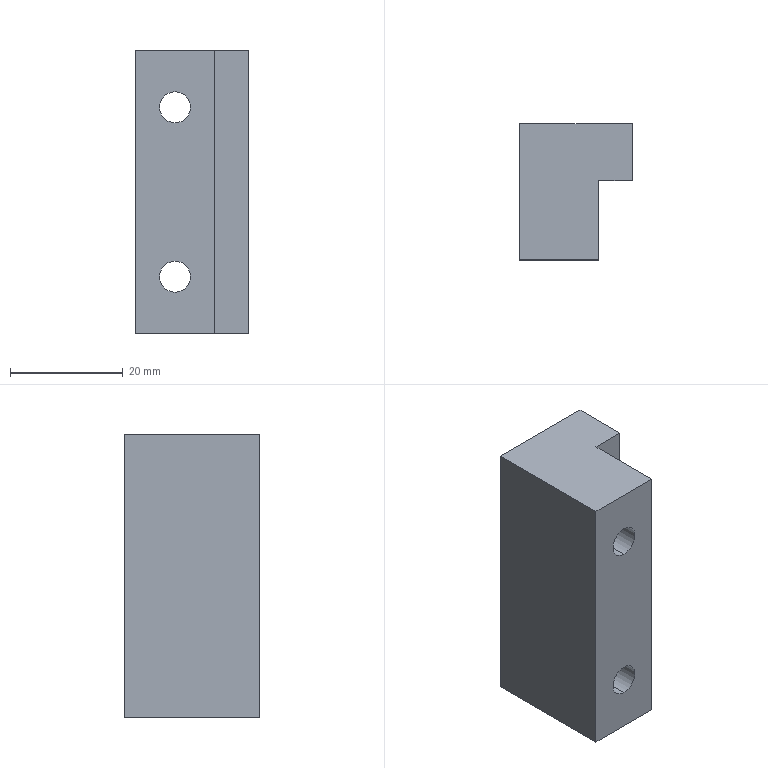Part | STEP file | Large cylinder connector mounting block | 1 solid | 18 faces | box 20 x 24 x 50 mm | volume 18141 mm3 | plane 10 | cylinder 8 | commonest cylinder face diameters 5.5 x4 9.5 x4
STEP:
#1=CARTESIAN_POINT('',(0.,0.,0.));
#2=DIRECTION('',(0.,0.,1.));
#3=DIRECTION('',(1.,0.,0.));
#4=AXIS2_PLACEMENT_3D('',#1,#2,#3);
#5=CARTESIAN_POINT('',(-13.,18.5,14.75));
#6=VERTEX_POINT('',#5);
#7=CARTESIAN_POINT('',(-13.,24.,14.75));
#8=VERTEX_POINT('',#7);
#9=CARTESIAN_POINT('',(-13.,24.,14.75));
#10=DIRECTION('',(0.,1.,0.));
#11=VECTOR('',#10,1.);
#12=LINE('',#9,#11);
#13=CARTESIAN_POINT('',(-13.,24.,10.));
#14=DIRECTION('',(0.,1.,0.));
#15=DIRECTION('',(0.,0.,1.));
#16=AXIS2_PLACEMENT_3D('',#13,#14,#15);
#17=CYLINDRICAL_SURFACE('',#16,4.75);
#18=CARTESIAN_POINT('',(6.283,0.));
#19=DIRECTION('',(0.,1.));
#20=VECTOR('',#19,1.);
#21=LINE('',#18,#20);
#22=(GEOMETRIC_REPRESENTATION_CONTEXT(2)PARAMETRIC_REPRESENTATION_CONTEXT()REPRESENTATION_CONTEXT('',''));
#23=DEFINITIONAL_REPRESENTATION('',(#21),#22);
#24=PCURVE('',#17,#23);
#25=CARTESIAN_POINT('',(-13.,24.,10.));
#26=DIRECTION('',(0.,1.,0.));
#27=DIRECTION('',(0.,0.,1.));
#28=AXIS2_PLACEMENT_3D('',#25,#26,#27);
#29=CYLINDRICAL_SURFACE('',#28,4.75);
#30=CARTESIAN_POINT('',(0.,0.));
#31=DIRECTION('',(0.,1.));
#32=VECTOR('',#31,1.);
#33=LINE('',#30,#32);
#34=(GEOMETRIC_REPRESENTATION_CONTEXT(2)PARAMETRIC_REPRESENTATION_CONTEXT()REPRESENTATION_CONTEXT('',''));
#35=DEFINITIONAL_REPRESENTATION('',(#33),#34);
#36=PCURVE('',#29,#35);
#37=SURFACE_CURVE('',#12,(#24,#36),.PCURVE_S1.);
#38=EDGE_CURVE('',#6,#8,#37,.T.);
#39=ORIENTED_EDGE('',*,*,#38,.T.);
#40=CARTESIAN_POINT('',(-13.,24.,5.25));
#41=VERTEX_POINT('',#40);
#42=CARTESIAN_POINT('',(-13.,24.,10.));
#43=DIRECTION('',(0.,1.,0.));
#44=DIRECTION('',(0.,0.,1.));
#45=AXIS2_PLACEMENT_3D('',#42,#43,#44);
#46=CIRCLE('',#45,4.75);
#47=CARTESIAN_POINT('',(0.,0.));
#48=DIRECTION('',(1.,0.));
#49=VECTOR('',#48,1.);
#50=LINE('',#47,#49);
#51=(GEOMETRIC_REPRESENTATION_CONTEXT(2)PARAMETRIC_REPRESENTATION_CONTEXT()REPRESENTATION_CONTEXT('',''));
#52=DEFINITIONAL_REPRESENTATION('',(#50),#51);
#53=PCURVE('',#17,#52);
#54=CARTESIAN_POINT('',(0.,24.,50.));
#55=DIRECTION('',(0.,-1.,0.));
#56=DIRECTION('',(1.,0.,0.));
#57=AXIS2_PLACEMENT_3D('',#54,#55,#56);
#58=PLANE('',#57);
#59=CARTESIAN_POINT('',(-13.,-35.25));
#60=CARTESIAN_POINT('',(-4.773,-35.25));
#61=CARTESIAN_POINT('',(-8.886,-42.375));
#62=CARTESIAN_POINT('',(-13.,-49.5));
#63=CARTESIAN_POINT('',(-17.114,-42.375));
#64=CARTESIAN_POINT('',(-21.227,-35.25));
#65=CARTESIAN_POINT('',(-13.,-35.25));
#66=(BOUNDED_CURVE()B_SPLINE_CURVE(2,(#59,#60,#61,#62,#63,#64,#65),.UNSPECIFIED.,.T.,.F.)B_SPLINE_CURVE_WITH_KNOTS((1,2,2,2,2,1),(-2.094,0.,2.094,4.189,6.283,8.378),.UNSPECIFIED.)CURVE()GEOMETRIC_REPRESENTATION_ITEM()RATIONAL_B_SPLINE_CURVE((1.,0.5,1.,0.5,1.,0.5,1.))REPRESENTATION_ITEM(''));
#67=(GEOMETRIC_REPRESENTATION_CONTEXT(2)PARAMETRIC_REPRESENTATION_CONTEXT()REPRESENTATION_CONTEXT('',''));
#68=DEFINITIONAL_REPRESENTATION('',(#66),#67);
#69=PCURVE('',#58,#68);
#70=SURFACE_CURVE('',#46,(#53,#69),.PCURVE_S1.);
#71=EDGE_CURVE('',#41,#8,#70,.T.);
#72=ORIENTED_EDGE('',*,*,#71,.F.);
#73=CARTESIAN_POINT('',(-13.,18.5,5.25));
#74=VERTEX_POINT('',#73);
#75=CARTESIAN_POINT('',(-13.,24.,5.25));
#76=DIRECTION('',(0.,1.,0.));
#77=VECTOR('',#76,1.);
#78=LINE('',#75,#77);
#79=CARTESIAN_POINT('',(3.142,0.));
#80=DIRECTION('',(0.,1.));
#81=VECTOR('',#80,1.);
#82=LINE('',#79,#81);
#83=(GEOMETRIC_REPRESENTATION_CONTEXT(2)PARAMETRIC_REPRESENTATION_CONTEXT()REPRESENTATION_CONTEXT('',''));
#84=DEFINITIONAL_REPRESENTATION('',(#82),#83);
#85=PCURVE('',#17,#84);
#86=CARTESIAN_POINT('',(3.142,0.));
#87=DIRECTION('',(0.,1.));
#88=VECTOR('',#87,1.);
#89=LINE('',#86,#88);
#90=(GEOMETRIC_REPRESENTATION_CONTEXT(2)PARAMETRIC_REPRESENTATION_CONTEXT()REPRESENTATION_CONTEXT('',''));
#91=DEFINITIONAL_REPRESENTATION('',(#89),#90);
#92=PCURVE('',#29,#91);
#93=SURFACE_CURVE('',#78,(#85,#92),.PCURVE_S1.);
#94=EDGE_CURVE('',#74,#41,#93,.T.);
#95=ORIENTED_EDGE('',*,*,#94,.F.);
#96=CARTESIAN_POINT('',(-13.,18.5,10.));
#97=DIRECTION('',(0.,1.,0.));
#98=DIRECTION('',(0.,0.,1.));
#99=AXIS2_PLACEMENT_3D('',#96,#97,#98);
#100=CIRCLE('',#99,4.75);
#101=CARTESIAN_POINT('',(0.,-5.5));
#102=DIRECTION('',(1.,0.));
#103=VECTOR('',#102,1.);
#104=LINE('',#101,#103);
#105=(GEOMETRIC_REPRESENTATION_CONTEXT(2)PARAMETRIC_REPRESENTATION_CONTEXT()REPRESENTATION_CONTEXT('',''));
#106=DEFINITIONAL_REPRESENTATION('',(#104),#105);
#107=PCURVE('',#17,#106);
#108=CARTESIAN_POINT('',(-10.25,18.5,10.));
#109=DIRECTION('',(0.,-1.,0.));
#110=DIRECTION('',(0.,0.,-1.));
#111=AXIS2_PLACEMENT_3D('',#108,#109,#110);
#112=PLANE('',#111);
#113=CARTESIAN_POINT('',(-4.75,-2.75));
#114=CARTESIAN_POINT('',(-4.75,5.477));
#115=CARTESIAN_POINT('',(2.375,1.364));
#116=CARTESIAN_POINT('',(9.5,-2.75));
#117=CARTESIAN_POINT('',(2.375,-6.864));
#118=CARTESIAN_POINT('',(-4.75,-10.977));
#119=CARTESIAN_POINT('',(-4.75,-2.75));
#120=(BOUNDED_CURVE()B_SPLINE_CURVE(2,(#113,#114,#115,#116,#117,#118,#119),.UNSPECIFIED.,.T.,.F.)B_SPLINE_CURVE_WITH_KNOTS((1,2,2,2,2,1),(-2.094,0.,2.094,4.189,6.283,8.378),.UNSPECIFIED.)CURVE()GEOMETRIC_REPRESENTATION_ITEM()RATIONAL_B_SPLINE_CURVE((1.,0.5,1.,0.5,1.,0.5,1.))REPRESENTATION_ITEM(''));
#121=(GEOMETRIC_REPRESENTATION_CONTEXT(2)PARAMETRIC_REPRESENTATION_CONTEXT()REPRESENTATION_CONTEXT('',''));
#122=DEFINITIONAL_REPRESENTATION('',(#120),#121);
#123=PCURVE('',#112,#122);
#124=SURFACE_CURVE('',#100,(#107,#123),.PCURVE_S1.);
#125=EDGE_CURVE('',#74,#6,#124,.T.);
#126=ORIENTED_EDGE('',*,*,#125,.T.);
#127=EDGE_LOOP('',(#39,#72,#95,#126));
#128=FACE_BOUND('',#127,.F.);
#129=ADVANCED_FACE('',(#128),#17,.F.);
#130=CARTESIAN_POINT('',(-13.,0.,12.75));
#131=VERTEX_POINT('',#130);
#132=CARTESIAN_POINT('',(-13.,18.5,12.75));
#133=VERTEX_POINT('',#132);
#134=CARTESIAN_POINT('',(-13.,24.,12.75));
#135=DIRECTION('',(0.,1.,0.));
#136=VECTOR('',#135,1.);
#137=LINE('',#134,#136);
#138=CARTESIAN_POINT('',(-13.,24.,10.));
#139=DIRECTION('',(0.,1.,0.));
#140=DIRECTION('',(0.,0.,1.));
#141=AXIS2_PLACEMENT_3D('',#138,#139,#140);
#142=CYLINDRICAL_SURFACE('',#141,2.75);
#143=CARTESIAN_POINT('',(6.283,0.));
#144=DIRECTION('',(0.,1.));
#145=VECTOR('',#144,1.);
#146=LINE('',#143,#145);
#147=(GEOMETRIC_REPRESENTATION_CONTEXT(2)PARAMETRIC_REPRESENTATION_CONTEXT()REPRESENTATION_CONTEXT('',''));
#148=DEFINITIONAL_REPRESENTATION('',(#146),#147);
#149=PCURVE('',#142,#148);
#150=CARTESIAN_POINT('',(-13.,24.,10.));
#151=DIRECTION('',(0.,1.,0.));
#152=DIRECTION('',(0.,0.,1.));
#153=AXIS2_PLACEMENT_3D('',#150,#151,#152);
#154=CYLINDRICAL_SURFACE('',#153,2.75);
#155=CARTESIAN_POINT('',(0.,0.));
#156=DIRECTION('',(0.,1.));
#157=VECTOR('',#156,1.);
#158=LINE('',#155,#157);
#159=(GEOMETRIC_REPRESENTATION_CONTEXT(2)PARAMETRIC_REPRESENTATION_CONTEXT()REPRESENTATION_CONTEXT('',''));
#160=DEFINITIONAL_REPRESENTATION('',(#158),#159);
#161=PCURVE('',#154,#160);
#162=SURFACE_CURVE('',#137,(#149,#161),.PCURVE_S1.);
#163=EDGE_CURVE('',#131,#133,#162,.T.);
#164=ORIENTED_EDGE('',*,*,#163,.T.);
#165=CARTESIAN_POINT('',(-13.,18.5,7.25));
#166=VERTEX_POINT('',#165);
#167=CARTESIAN_POINT('',(-13.,18.5,10.));
#168=DIRECTION('',(0.,1.,0.));
#169=DIRECTION('',(0.,0.,1.));
#170=AXIS2_PLACEMENT_3D('',#167,#168,#169);
#171=CIRCLE('',#170,2.75);
#172=CARTESIAN_POINT('',(0.,-5.5));
#173=DIRECTION('',(1.,0.));
#174=VECTOR('',#173,1.);
#175=LINE('',#172,#174);
#176=(GEOMETRIC_REPRESENTATION_CONTEXT(2)PARAMETRIC_REPRESENTATION_CONTEXT()REPRESENTATION_CONTEXT('',''));
#177=DEFINITIONAL_REPRESENTATION('',(#175),#176);
#178=PCURVE('',#142,#177);
#179=CARTESIAN_POINT('',(-2.75,-2.75));
#180=CARTESIAN_POINT('',(-2.75,2.013));
#181=CARTESIAN_POINT('',(1.375,-0.3684));
#182=CARTESIAN_POINT('',(5.5,-2.75));
#183=CARTESIAN_POINT('',(1.375,-5.132));
#184=CARTESIAN_POINT('',(-2.75,-7.513));
#185=CARTESIAN_POINT('',(-2.75,-2.75));
#186=(BOUNDED_CURVE()B_SPLINE_CURVE(2,(#179,#180,#181,#182,#183,#184,#185),.UNSPECIFIED.,.T.,.F.)B_SPLINE_CURVE_WITH_KNOTS((1,2,2,2,2,1),(-2.094,0.,2.094,4.189,6.283,8.378),.UNSPECIFIED.)CURVE()GEOMETRIC_REPRESENTATION_ITEM()RATIONAL_B_SPLINE_CURVE((1.,0.5,1.,0.5,1.,0.5,1.))REPRESENTATION_ITEM(''));
#187=(GEOMETRIC_REPRESENTATION_CONTEXT(2)PARAMETRIC_REPRESENTATION_CONTEXT()REPRESENTATION_CONTEXT('',''));
#188=DEFINITIONAL_REPRESENTATION('',(#186),#187);
#189=PCURVE('',#112,#188);
#190=SURFACE_CURVE('',#171,(#178,#189),.PCURVE_S1.);
#191=EDGE_CURVE('',#166,#133,#190,.T.);
#192=ORIENTED_EDGE('',*,*,#191,.F.);
#193=CARTESIAN_POINT('',(-13.,0.,7.25));
#194=VERTEX_POINT('',#193);
#195=CARTESIAN_POINT('',(-13.,24.,7.25));
#196=DIRECTION('',(0.,1.,0.));
#197=VECTOR('',#196,1.);
#198=LINE('',#195,#197);
#199=CARTESIAN_POINT('',(3.142,0.));
#200=DIRECTION('',(0.,1.));
#201=VECTOR('',#200,1.);
#202=LINE('',#199,#201);
#203=(GEOMETRIC_REPRESENTATION_CONTEXT(2)PARAMETRIC_REPRESENTATION_CONTEXT()REPRESENTATION_CONTEXT('',''));
#204=DEFINITIONAL_REPRESENTATION('',(#202),#203);
#205=PCURVE('',#142,#204);
#206=CARTESIAN_POINT('',(3.142,0.));
#207=DIRECTION('',(0.,1.));
#208=VECTOR('',#207,1.);
#209=LINE('',#206,#208);
#210=(GEOMETRIC_REPRESENTATION_CONTEXT(2)PARAMETRIC_REPRESENTATION_CONTEXT()REPRESENTATION_CONTEXT('',''));
#211=DEFINITIONAL_REPRESENTATION('',(#209),#210);
#212=PCURVE('',#154,#211);
#213=SURFACE_CURVE('',#198,(#205,#212),.PCURVE_S1.);
#214=EDGE_CURVE('',#194,#166,#213,.T.);
#215=ORIENTED_EDGE('',*,*,#214,.F.);
#216=CARTESIAN_POINT('',(-13.,0.,10.));
#217=DIRECTION('',(0.,1.,0.));
#218=DIRECTION('',(-1.,0.,0.));
#219=AXIS2_PLACEMENT_3D('',#216,#217,#218);
#220=CIRCLE('',#219,2.75);
#221=CARTESIAN_POINT('',(-1.571,-24.));
#222=DIRECTION('',(1.,0.));
#223=VECTOR('',#222,1.);
#224=LINE('',#221,#223);
#225=(GEOMETRIC_REPRESENTATION_CONTEXT(2)PARAMETRIC_REPRESENTATION_CONTEXT()REPRESENTATION_CONTEXT('',''));
#226=DEFINITIONAL_REPRESENTATION('',(#224),#225);
#227=PCURVE('',#142,#226);
#228=CARTESIAN_POINT('',(0.,0.,50.));
#229=DIRECTION('',(0.,1.,0.));
#230=DIRECTION('',(-1.,0.,0.));
#231=AXIS2_PLACEMENT_3D('',#228,#229,#230);
#232=PLANE('',#231);
#233=CARTESIAN_POINT('',(13.,-40.));
#234=DIRECTION('',(1.,0.));
#235=AXIS2_PLACEMENT_2D('',#233,#234);
#236=CIRCLE('',#235,2.75);
#237=(GEOMETRIC_REPRESENTATION_CONTEXT(2)PARAMETRIC_REPRESENTATION_CONTEXT()REPRESENTATION_CONTEXT('',''));
#238=DEFINITIONAL_REPRESENTATION('',(#236),#237);
#239=PCURVE('',#232,#238);
#240=SURFACE_CURVE('',#220,(#227,#239),.PCURVE_S1.);
#241=EDGE_CURVE('',#194,#131,#240,.T.);
#242=ORIENTED_EDGE('',*,*,#241,.T.);
#243=EDGE_LOOP('',(#164,#192,#215,#242));
#244=FACE_BOUND('',#243,.F.);
#245=ADVANCED_FACE('',(#244),#142,.F.);
#246=CARTESIAN_POINT('',(-13.,18.5,44.75));
#247=VERTEX_POINT('',#246);
#248=CARTESIAN_POINT('',(-13.,24.,44.75));
#249=VERTEX_POINT('',#248);
#250=CARTESIAN_POINT('',(-13.,24.,44.75));
#251=DIRECTION('',(0.,1.,0.));
#252=VECTOR('',#251,1.);
#253=LINE('',#250,#252);
#254=CARTESIAN_POINT('',(-13.,24.,40.));
#255=DIRECTION('',(0.,1.,0.));
#256=DIRECTION('',(0.,0.,1.));
#257=AXIS2_PLACEMENT_3D('',#254,#255,#256);
#258=CYLINDRICAL_SURFACE('',#257,4.75);
#259=CARTESIAN_POINT('',(6.283,0.));
#260=DIRECTION('',(0.,1.));
#261=VECTOR('',#260,1.);
#262=LINE('',#259,#261);
#263=(GEOMETRIC_REPRESENTATION_CONTEXT(2)PARAMETRIC_REPRESENTATION_CONTEXT()REPRESENTATION_CONTEXT('',''));
#264=DEFINITIONAL_REPRESENTATION('',(#262),#263);
#265=PCURVE('',#258,#264);
#266=CARTESIAN_POINT('',(-13.,24.,40.));
#267=DIRECTION('',(0.,1.,0.));
#268=DIRECTION('',(0.,0.,1.));
#269=AXIS2_PLACEMENT_3D('',#266,#267,#268);
#270=CYLINDRICAL_SURFACE('',#269,4.75);
#271=CARTESIAN_POINT('',(0.,0.));
#272=DIRECTION('',(0.,1.));
#273=VECTOR('',#272,1.);
#274=LINE('',#271,#273);
#275=(GEOMETRIC_REPRESENTATION_CONTEXT(2)PARAMETRIC_REPRESENTATION_CONTEXT()REPRESENTATION_CONTEXT('',''));
#276=DEFINITIONAL_REPRESENTATION('',(#274),#275);
#277=PCURVE('',#270,#276);
#278=SURFACE_CURVE('',#253,(#265,#277),.PCURVE_S1.);
#279=EDGE_CURVE('',#247,#249,#278,.T.);
#280=ORIENTED_EDGE('',*,*,#279,.T.);
#281=CARTESIAN_POINT('',(-13.,24.,35.25));
#282=VERTEX_POINT('',#281);
#283=CARTESIAN_POINT('',(-13.,24.,40.));
#284=DIRECTION('',(0.,1.,0.));
#285=DIRECTION('',(0.,0.,1.));
#286=AXIS2_PLACEMENT_3D('',#283,#284,#285);
#287=CIRCLE('',#286,4.75);
#288=CARTESIAN_POINT('',(0.,0.));
#289=DIRECTION('',(1.,0.));
#290=VECTOR('',#289,1.);
#291=LINE('',#288,#290);
#292=(GEOMETRIC_REPRESENTATION_CONTEXT(2)PARAMETRIC_REPRESENTATION_CONTEXT()REPRESENTATION_CONTEXT('',''));
#293=DEFINITIONAL_REPRESENTATION('',(#291),#292);
#294=PCURVE('',#258,#293);
#295=CARTESIAN_POINT('',(-13.,-5.25));
#296=CARTESIAN_POINT('',(-4.773,-5.25));
#297=CARTESIAN_POINT('',(-8.886,-12.375));
#298=CARTESIAN_POINT('',(-13.,-19.5));
#299=CARTESIAN_POINT('',(-17.114,-12.375));
#300=CARTESIAN_POINT('',(-21.227,-5.25));
#301=CARTESIAN_POINT('',(-13.,-5.25));
#302=(BOUNDED_CURVE()B_SPLINE_CURVE(2,(#295,#296,#297,#298,#299,#300,#301),.UNSPECIFIED.,.T.,.F.)B_SPLINE_CURVE_WITH_KNOTS((1,2,2,2,2,1),(-2.094,0.,2.094,4.189,6.283,8.378),.UNSPECIFIED.)CURVE()GEOMETRIC_REPRESENTATION_ITEM()RATIONAL_B_SPLINE_CURVE((1.,0.5,1.,0.5,1.,0.5,1.))REPRESENTATION_ITEM(''));
#303=(GEOMETRIC_REPRESENTATION_CONTEXT(2)PARAMETRIC_REPRESENTATION_CONTEXT()REPRESENTATION_CONTEXT('',''));
#304=DEFINITIONAL_REPRESENTATION('',(#302),#303);
#305=PCURVE('',#58,#304);
#306=SURFACE_CURVE('',#287,(#294,#305),.PCURVE_S1.);
#307=EDGE_CURVE('',#282,#249,#306,.T.);
#308=ORIENTED_EDGE('',*,*,#307,.F.);
#309=CARTESIAN_POINT('',(-13.,18.5,35.25));
#310=VERTEX_POINT('',#309);
#311=CARTESIAN_POINT('',(-13.,24.,35.25));
#312=DIRECTION('',(0.,1.,0.));
#313=VECTOR('',#312,1.);
#314=LINE('',#311,#313);
#315=CARTESIAN_POINT('',(3.142,0.));
#316=DIRECTION('',(0.,1.));
#317=VECTOR('',#316,1.);
#318=LINE('',#315,#317);
#319=(GEOMETRIC_REPRESENTATION_CONTEXT(2)PARAMETRIC_REPRESENTATION_CONTEXT()REPRESENTATION_CONTEXT('',''));
#320=DEFINITIONAL_REPRESENTATION('',(#318),#319);
#321=PCURVE('',#258,#320);
#322=CARTESIAN_POINT('',(3.142,0.));
#323=DIRECTION('',(0.,1.));
#324=VECTOR('',#323,1.);
#325=LINE('',#322,#324);
#326=(GEOMETRIC_REPRESENTATION_CONTEXT(2)PARAMETRIC_REPRESENTATION_CONTEXT()REPRESENTATION_CONTEXT('',''));
#327=DEFINITIONAL_REPRESENTATION('',(#325),#326);
#328=PCURVE('',#270,#327);
#329=SURFACE_CURVE('',#314,(#321,#328),.PCURVE_S1.);
#330=EDGE_CURVE('',#310,#282,#329,.T.);
#331=ORIENTED_EDGE('',*,*,#330,.F.);
#332=CARTESIAN_POINT('',(-13.,18.5,40.));
#333=DIRECTION('',(0.,1.,0.));
#334=DIRECTION('',(0.,0.,1.));
#335=AXIS2_PLACEMENT_3D('',#332,#333,#334);
#336=CIRCLE('',#335,4.75);
#337=CARTESIAN_POINT('',(0.,-5.5));
#338=DIRECTION('',(1.,0.));
#339=VECTOR('',#338,1.);
#340=LINE('',#337,#339);
#341=(GEOMETRIC_REPRESENTATION_CONTEXT(2)PARAMETRIC_REPRESENTATION_CONTEXT()REPRESENTATION_CONTEXT('',''));
#342=DEFINITIONAL_REPRESENTATION('',(#340),#341);
#343=PCURVE('',#258,#342);
#344=CARTESIAN_POINT('',(-10.25,18.5,40.));
#345=DIRECTION('',(0.,-1.,0.));
#346=DIRECTION('',(0.,0.,-1.));
#347=AXIS2_PLACEMENT_3D('',#344,#345,#346);
#348=PLANE('',#347);
#349=CARTESIAN_POINT('',(-4.75,-2.75));
#350=CARTESIAN_POINT('',(-4.75,5.477));
#351=CARTESIAN_POINT('',(2.375,1.364));
#352=CARTESIAN_POINT('',(9.5,-2.75));
#353=CARTESIAN_POINT('',(2.375,-6.864));
#354=CARTESIAN_POINT('',(-4.75,-10.977));
#355=CARTESIAN_POINT('',(-4.75,-2.75));
#356=(BOUNDED_CURVE()B_SPLINE_CURVE(2,(#349,#350,#351,#352,#353,#354,#355),.UNSPECIFIED.,.T.,.F.)B_SPLINE_CURVE_WITH_KNOTS((1,2,2,2,2,1),(-2.094,0.,2.094,4.189,6.283,8.378),.UNSPECIFIED.)CURVE()GEOMETRIC_REPRESENTATION_ITEM()RATIONAL_B_SPLINE_CURVE((1.,0.5,1.,0.5,1.,0.5,1.))REPRESENTATION_ITEM(''));
#357=(GEOMETRIC_REPRESENTATION_CONTEXT(2)PARAMETRIC_REPRESENTATION_CONTEXT()REPRESENTATION_CONTEXT('',''));
#358=DEFINITIONAL_REPRESENTATION('',(#356),#357);
#359=PCURVE('',#348,#358);
#360=SURFACE_CURVE('',#336,(#343,#359),.PCURVE_S1.);
#361=EDGE_CURVE('',#310,#247,#360,.T.);
#362=ORIENTED_EDGE('',*,*,#361,.T.);
#363=EDGE_LOOP('',(#280,#308,#331,#362));
#364=FACE_BOUND('',#363,.F.);
#365=ADVANCED_FACE('',(#364),#258,.F.);
#366=CARTESIAN_POINT('',(-13.,0.,42.75));
#367=VERTEX_POINT('',#366);
#368=CARTESIAN_POINT('',(-13.,18.5,42.75));
#369=VERTEX_POINT('',#368);
#370=CARTESIAN_POINT('',(-13.,24.,42.75));
#371=DIRECTION('',(0.,1.,0.));
#372=VECTOR('',#371,1.);
#373=LINE('',#370,#372);
#374=CARTESIAN_POINT('',(-13.,24.,40.));
#375=DIRECTION('',(0.,1.,0.));
#376=DIRECTION('',(0.,0.,1.));
#377=AXIS2_PLACEMENT_3D('',#374,#375,#376);
#378=CYLINDRICAL_SURFACE('',#377,2.75);
#379=CARTESIAN_POINT('',(6.283,0.));
#380=DIRECTION('',(0.,1.));
#381=VECTOR('',#380,1.);
#382=LINE('',#379,#381);
#383=(GEOMETRIC_REPRESENTATION_CONTEXT(2)PARAMETRIC_REPRESENTATION_CONTEXT()REPRESENTATION_CONTEXT('',''));
#384=DEFINITIONAL_REPRESENTATION('',(#382),#383);
#385=PCURVE('',#378,#384);
#386=CARTESIAN_POINT('',(-13.,24.,40.));
#387=DIRECTION('',(0.,1.,0.));
#388=DIRECTION('',(0.,0.,1.));
#389=AXIS2_PLACEMENT_3D('',#386,#387,#388);
#390=CYLINDRICAL_SURFACE('',#389,2.75);
#391=CARTESIAN_POINT('',(0.,0.));
#392=DIRECTION('',(0.,1.));
#393=VECTOR('',#392,1.);
#394=LINE('',#391,#393);
#395=(GEOMETRIC_REPRESENTATION_CONTEXT(2)PARAMETRIC_REPRESENTATION_CONTEXT()REPRESENTATION_CONTEXT('',''));
#396=DEFINITIONAL_REPRESENTATION('',(#394),#395);
#397=PCURVE('',#390,#396);
#398=SURFACE_CURVE('',#373,(#385,#397),.PCURVE_S1.);
#399=EDGE_CURVE('',#367,#369,#398,.T.);
#400=ORIENTED_EDGE('',*,*,#399,.T.);
#401=CARTESIAN_POINT('',(-13.,18.5,37.25));
#402=VERTEX_POINT('',#401);
#403=CARTESIAN_POINT('',(-13.,18.5,40.));
#404=DIRECTION('',(0.,1.,0.));
#405=DIRECTION('',(0.,0.,1.));
#406=AXIS2_PLACEMENT_3D('',#403,#404,#405);
#407=CIRCLE('',#406,2.75);
#408=CARTESIAN_POINT('',(0.,-5.5));
#409=DIRECTION('',(1.,0.));
#410=VECTOR('',#409,1.);
#411=LINE('',#408,#410);
#412=(GEOMETRIC_REPRESENTATION_CONTEXT(2)PARAMETRIC_REPRESENTATION_CONTEXT()REPRESENTATION_CONTEXT('',''));
#413=DEFINITIONAL_REPRESENTATION('',(#411),#412);
#414=PCURVE('',#378,#413);
#415=CARTESIAN_POINT('',(-2.75,-2.75));
#416=CARTESIAN_POINT('',(-2.75,2.013));
#417=CARTESIAN_POINT('',(1.375,-0.3684));
#418=CARTESIAN_POINT('',(5.5,-2.75));
#419=CARTESIAN_POINT('',(1.375,-5.132));
#420=CARTESIAN_POINT('',(-2.75,-7.513));
#421=CARTESIAN_POINT('',(-2.75,-2.75));
#422=(BOUNDED_CURVE()B_SPLINE_CURVE(2,(#415,#416,#417,#418,#419,#420,#421),.UNSPECIFIED.,.T.,.F.)B_SPLINE_CURVE_WITH_KNOTS((1,2,2,2,2,1),(-2.094,0.,2.094,4.189,6.283,8.378),.UNSPECIFIED.)CURVE()GEOMETRIC_REPRESENTATION_ITEM()RATIONAL_B_SPLINE_CURVE((1.,0.5,1.,0.5,1.,0.5,1.))REPRESENTATION_ITEM(''));
#423=(GEOMETRIC_REPRESENTATION_CONTEXT(2)PARAMETRIC_REPRESENTATION_CONTEXT()REPRESENTATION_CONTEXT('',''));
#424=DEFINITIONAL_REPRESENTATION('',(#422),#423);
#425=PCURVE('',#348,#424);
#426=SURFACE_CURVE('',#407,(#414,#425),.PCURVE_S1.);
#427=EDGE_CURVE('',#402,#369,#426,.T.);
#428=ORIENTED_EDGE('',*,*,#427,.F.);
#429=CARTESIAN_POINT('',(-13.,0.,37.25));
#430=VERTEX_POINT('',#429);
#431=CARTESIAN_POINT('',(-13.,24.,37.25));
#432=DIRECTION('',(0.,1.,0.));
#433=VECTOR('',#432,1.);
#434=LINE('',#431,#433);
#435=CARTESIAN_POINT('',(3.142,0.));
#436=DIRECTION('',(0.,1.));
#437=VECTOR('',#436,1.);
#438=LINE('',#435,#437);
#439=(GEOMETRIC_REPRESENTATION_CONTEXT(2)PARAMETRIC_REPRESENTATION_CONTEXT()REPRESENTATION_CONTEXT('',''));
#440=DEFINITIONAL_REPRESENTATION('',(#438),#439);
#441=PCURVE('',#378,#440);
#442=CARTESIAN_POINT('',(3.142,0.));
#443=DIRECTION('',(0.,1.));
#444=VECTOR('',#443,1.);
#445=LINE('',#442,#444);
#446=(GEOMETRIC_REPRESENTATION_CONTEXT(2)PARAMETRIC_REPRESENTATION_CONTEXT()REPRESENTATION_CONTEXT('',''));
#447=DEFINITIONAL_REPRESENTATION('',(#445),#446);
#448=PCURVE('',#390,#447);
#449=SURFACE_CURVE('',#434,(#441,#448),.PCURVE_S1.);
#450=EDGE_CURVE('',#430,#402,#449,.T.);
#451=ORIENTED_EDGE('',*,*,#450,.F.);
#452=CARTESIAN_POINT('',(-13.,0.,40.));
#453=DIRECTION('',(0.,1.,0.));
#454=DIRECTION('',(-1.,0.,0.));
#455=AXIS2_PLACEMENT_3D('',#452,#453,#454);
#456=CIRCLE('',#455,2.75);
#457=CARTESIAN_POINT('',(-1.571,-24.));
#458=DIRECTION('',(1.,0.));
#459=VECTOR('',#458,1.);
#460=LINE('',#457,#459);
#461=(GEOMETRIC_REPRESENTATION_CONTEXT(2)PARAMETRIC_REPRESENTATION_CONTEXT()REPRESENTATION_CONTEXT('',''));
#462=DEFINITIONAL_REPRESENTATION('',(#460),#461);
#463=PCURVE('',#378,#462);
#464=CARTESIAN_POINT('',(13.,-10.));
#465=DIRECTION('',(1.,0.));
#466=AXIS2_PLACEMENT_2D('',#464,#465);
#467=CIRCLE('',#466,2.75);
#468=(GEOMETRIC_REPRESENTATION_CONTEXT(2)PARAMETRIC_REPRESENTATION_CONTEXT()REPRESENTATION_CONTEXT('',''));
#469=DEFINITIONAL_REPRESENTATION('',(#467),#468);
#470=PCURVE('',#232,#469);
#471=SURFACE_CURVE('',#456,(#463,#470),.PCURVE_S1.);
#472=EDGE_CURVE('',#430,#367,#471,.T.);
#473=ORIENTED_EDGE('',*,*,#472,.T.);
#474=EDGE_LOOP('',(#400,#428,#451,#473));
#475=FACE_BOUND('',#474,.F.);
#476=ADVANCED_FACE('',(#475),#378,.F.);
#477=CARTESIAN_POINT('',(0.,14.,50.));
#478=VERTEX_POINT('',#477);
#479=CARTESIAN_POINT('',(0.,24.,50.));
#480=VERTEX_POINT('',#479);
#481=CARTESIAN_POINT('',(0.,0.,50.));
#482=DIRECTION('',(0.,1.,0.));
#483=VECTOR('',#482,1.);
#484=LINE('',#481,#483);
#485=CARTESIAN_POINT('',(0.,0.,50.));
#486=DIRECTION('',(-1.,0.,0.));
#487=DIRECTION('',(0.,0.,1.));
#488=AXIS2_PLACEMENT_3D('',#485,#486,#487);
#489=PLANE('',#488);
#490=CARTESIAN_POINT('',(0.,0.));
#491=DIRECTION('',(0.,1.));
#492=VECTOR('',#491,1.);
#493=LINE('',#490,#492);
#494=(GEOMETRIC_REPRESENTATION_CONTEXT(2)PARAMETRIC_REPRESENTATION_CONTEXT()REPRESENTATION_CONTEXT('',''));
#495=DEFINITIONAL_REPRESENTATION('',(#493),#494);
#496=PCURVE('',#489,#495);
#497=CARTESIAN_POINT('',(0.,24.,50.));
#498=DIRECTION('',(0.,0.,1.));
#499=DIRECTION('',(1.,0.,0.));
#500=AXIS2_PLACEMENT_3D('',#497,#498,#499);
#501=PLANE('',#500);
#502=CARTESIAN_POINT('',(0.,-24.));
#503=DIRECTION('',(0.,1.));
#504=VECTOR('',#503,1.);
#505=LINE('',#502,#504);
#506=(GEOMETRIC_REPRESENTATION_CONTEXT(2)PARAMETRIC_REPRESENTATION_CONTEXT()REPRESENTATION_CONTEXT('',''));
#507=DEFINITIONAL_REPRESENTATION('',(#505),#506);
#508=PCURVE('',#501,#507);
#509=SURFACE_CURVE('',#484,(#496,#508),.PCURVE_S1.);
#510=EDGE_CURVE('',#478,#480,#509,.T.);
#511=ORIENTED_EDGE('',*,*,#510,.F.);
#512=CARTESIAN_POINT('',(0.,14.,0.));
#513=VERTEX_POINT('',#512);
#514=CARTESIAN_POINT('',(0.,14.,50.));
#515=DIRECTION('',(0.,0.,-1.));
#516=VECTOR('',#515,1.);
#517=LINE('',#514,#516);
#518=CARTESIAN_POINT('',(0.,14.));
#519=DIRECTION('',(-1.,0.));
#520=VECTOR('',#519,1.);
#521=LINE('',#518,#520);
#522=(GEOMETRIC_REPRESENTATION_CONTEXT(2)PARAMETRIC_REPRESENTATION_CONTEXT()REPRESENTATION_CONTEXT('',''));
#523=DEFINITIONAL_REPRESENTATION('',(#521),#522);
#524=PCURVE('',#489,#523);
#525=CARTESIAN_POINT('',(16.115,14.,0.));
#526=DIRECTION('',(0.,1.,0.));
#527=DIRECTION('',(-1.,0.,0.));
#528=AXIS2_PLACEMENT_3D('',#525,#526,#527);
#529=PLANE('',#528);
#530=CARTESIAN_POINT('',(16.115,50.));
#531=DIRECTION('',(0.,-1.));
#532=VECTOR('',#531,1.);
#533=LINE('',#530,#532);
#534=(GEOMETRIC_REPRESENTATION_CONTEXT(2)PARAMETRIC_REPRESENTATION_CONTEXT()REPRESENTATION_CONTEXT('',''));
#535=DEFINITIONAL_REPRESENTATION('',(#533),#534);
#536=PCURVE('',#529,#535);
#537=SURFACE_CURVE('',#517,(#524,#536),.PCURVE_S1.);
#538=EDGE_CURVE('',#478,#513,#537,.T.);
#539=ORIENTED_EDGE('',*,*,#538,.T.);
#540=CARTESIAN_POINT('',(0.,24.,0.));
#541=VERTEX_POINT('',#540);
#542=CARTESIAN_POINT('',(0.,0.,0.));
#543=DIRECTION('',(0.,1.,0.));
#544=VECTOR('',#543,1.);
#545=LINE('',#542,#544);
#546=CARTESIAN_POINT('',(-50.,0.));
#547=DIRECTION('',(0.,1.));
#548=VECTOR('',#547,1.);
#549=LINE('',#546,#548);
#550=(GEOMETRIC_REPRESENTATION_CONTEXT(2)PARAMETRIC_REPRESENTATION_CONTEXT()REPRESENTATION_CONTEXT('',''));
#551=DEFINITIONAL_REPRESENTATION('',(#549),#550);
#552=PCURVE('',#489,#551);
#553=CARTESIAN_POINT('',(0.,24.,0.));
#554=DIRECTION('',(0.,0.,1.));
#555=DIRECTION('',(1.,0.,0.));
#556=AXIS2_PLACEMENT_3D('',#553,#554,#555);
#557=PLANE('',#556);
#558=CARTESIAN_POINT('',(0.,-24.));
#559=DIRECTION('',(0.,1.));
#560=VECTOR('',#559,1.);
#561=LINE('',#558,#560);
#562=(GEOMETRIC_REPRESENTATION_CONTEXT(2)PARAMETRIC_REPRESENTATION_CONTEXT()REPRESENTATION_CONTEXT('',''));
#563=DEFINITIONAL_REPRESENTATION('',(#561),#562);
#564=PCURVE('',#557,#563);
#565=SURFACE_CURVE('',#545,(#552,#564),.PCURVE_S1.);
#566=EDGE_CURVE('',#513,#541,#565,.T.);
#567=ORIENTED_EDGE('',*,*,#566,.T.);
#568=CARTESIAN_POINT('',(0.,24.,50.));
#569=DIRECTION('',(0.,0.,-1.));
#570=VECTOR('',#569,1.);
#571=LINE('',#568,#570);
#572=CARTESIAN_POINT('',(0.,24.));
#573=DIRECTION('',(-1.,0.));
#574=VECTOR('',#573,1.);
#575=LINE('',#572,#574);
#576=(GEOMETRIC_REPRESENTATION_CONTEXT(2)PARAMETRIC_REPRESENTATION_CONTEXT()REPRESENTATION_CONTEXT('',''));
#577=DEFINITIONAL_REPRESENTATION('',(#575),#576);
#578=PCURVE('',#489,#577);
#579=CARTESIAN_POINT('',(0.,0.));
#580=DIRECTION('',(0.,-1.));
#581=VECTOR('',#580,1.);
#582=LINE('',#579,#581);
#583=(GEOMETRIC_REPRESENTATION_CONTEXT(2)PARAMETRIC_REPRESENTATION_CONTEXT()REPRESENTATION_CONTEXT('',''));
#584=DEFINITIONAL_REPRESENTATION('',(#582),#583);
#585=PCURVE('',#58,#584);
#586=SURFACE_CURVE('',#571,(#578,#585),.PCURVE_S1.);
#587=EDGE_CURVE('',#480,#541,#586,.T.);
#588=ORIENTED_EDGE('',*,*,#587,.F.);
#589=EDGE_LOOP('',(#511,#539,#567,#588));
#590=FACE_BOUND('',#589,.T.);
#591=ADVANCED_FACE('',(#590),#489,.F.);
#592=CARTESIAN_POINT('',(-13.,24.,10.));
#593=DIRECTION('',(0.,1.,0.));
#594=DIRECTION('',(0.,0.,1.));
#595=AXIS2_PLACEMENT_3D('',#592,#593,#594);
#596=CIRCLE('',#595,4.75);
#597=CARTESIAN_POINT('',(-13.,-35.25));
#598=CARTESIAN_POINT('',(-4.773,-35.25));
#599=CARTESIAN_POINT('',(-8.886,-42.375));
#600=CARTESIAN_POINT('',(-13.,-49.5));
#601=CARTESIAN_POINT('',(-17.114,-42.375));
#602=CARTESIAN_POINT('',(-21.227,-35.25));
#603=CARTESIAN_POINT('',(-13.,-35.25));
#604=(BOUNDED_CURVE()B_SPLINE_CURVE(2,(#597,#598,#599,#600,#601,#602,#603),.UNSPECIFIED.,.T.,.F.)B_SPLINE_CURVE_WITH_KNOTS((1,2,2,2,2,1),(-2.094,0.,2.094,4.189,6.283,8.378),.UNSPECIFIED.)CURVE()GEOMETRIC_REPRESENTATION_ITEM()RATIONAL_B_SPLINE_CURVE((1.,0.5,1.,0.5,1.,0.5,1.))REPRESENTATION_ITEM(''));
#605=(GEOMETRIC_REPRESENTATION_CONTEXT(2)PARAMETRIC_REPRESENTATION_CONTEXT()REPRESENTATION_CONTEXT('',''));
#606=DEFINITIONAL_REPRESENTATION('',(#604),#605);
#607=PCURVE('',#58,#606);
#608=CARTESIAN_POINT('',(0.,0.));
#609=DIRECTION('',(1.,0.));
#610=VECTOR('',#609,1.);
#611=LINE('',#608,#610);
#612=(GEOMETRIC_REPRESENTATION_CONTEXT(2)PARAMETRIC_REPRESENTATION_CONTEXT()REPRESENTATION_CONTEXT('',''));
#613=DEFINITIONAL_REPRESENTATION('',(#611),#612);
#614=PCURVE('',#29,#613);
#615=SURFACE_CURVE('',#596,(#607,#614),.PCURVE_S1.);
#616=EDGE_CURVE('',#8,#41,#615,.T.);
#617=ORIENTED_EDGE('',*,*,#616,.F.);
#618=ORIENTED_EDGE('',*,*,#71,.F.);
#619=EDGE_LOOP('',(#617,#618));
#620=FACE_BOUND('',#619,.T.);
#621=CARTESIAN_POINT('',(-13.,24.,40.));
#622=DIRECTION('',(0.,1.,0.));
#623=DIRECTION('',(0.,0.,1.));
#624=AXIS2_PLACEMENT_3D('',#621,#622,#623);
#625=CIRCLE('',#624,4.75);
#626=CARTESIAN_POINT('',(-13.,-5.25));
#627=CARTESIAN_POINT('',(-4.773,-5.25));
#628=CARTESIAN_POINT('',(-8.886,-12.375));
#629=CARTESIAN_POINT('',(-13.,-19.5));
#630=CARTESIAN_POINT('',(-17.114,-12.375));
#631=CARTESIAN_POINT('',(-21.227,-5.25));
#632=CARTESIAN_POINT('',(-13.,-5.25));
#633=(BOUNDED_CURVE()B_SPLINE_CURVE(2,(#626,#627,#628,#629,#630,#631,#632),.UNSPECIFIED.,.T.,.F.)B_SPLINE_CURVE_WITH_KNOTS((1,2,2,2,2,1),(-2.094,0.,2.094,4.189,6.283,8.378),.UNSPECIFIED.)CURVE()GEOMETRIC_REPRESENTATION_ITEM()RATIONAL_B_SPLINE_CURVE((1.,0.5,1.,0.5,1.,0.5,1.))REPRESENTATION_ITEM(''));
#634=(GEOMETRIC_REPRESENTATION_CONTEXT(2)PARAMETRIC_REPRESENTATION_CONTEXT()REPRESENTATION_CONTEXT('',''));
#635=DEFINITIONAL_REPRESENTATION('',(#633),#634);
#636=PCURVE('',#58,#635);
#637=CARTESIAN_POINT('',(0.,0.));
#638=DIRECTION('',(1.,0.));
#639=VECTOR('',#638,1.);
#640=LINE('',#637,#639);
#641=(GEOMETRIC_REPRESENTATION_CONTEXT(2)PARAMETRIC_REPRESENTATION_CONTEXT()REPRESENTATION_CONTEXT('',''));
#642=DEFINITIONAL_REPRESENTATION('',(#640),#641);
#643=PCURVE('',#270,#642);
#644=SURFACE_CURVE('',#625,(#636,#643),.PCURVE_S1.);
#645=EDGE_CURVE('',#249,#282,#644,.T.);
#646=ORIENTED_EDGE('',*,*,#645,.F.);
#647=ORIENTED_EDGE('',*,*,#307,.F.);
#648=EDGE_LOOP('',(#646,#647));
#649=FACE_BOUND('',#648,.T.);
#650=CARTESIAN_POINT('',(-20.,24.,0.));
#651=VERTEX_POINT('',#650);
#652=CARTESIAN_POINT('',(0.,24.,0.));
#653=DIRECTION('',(-1.,0.,0.));
#654=VECTOR('',#653,1.);
#655=LINE('',#652,#654);
#656=CARTESIAN_POINT('',(0.,-50.));
#657=DIRECTION('',(-1.,0.));
#658=VECTOR('',#657,1.);
#659=LINE('',#656,#658);
#660=(GEOMETRIC_REPRESENTATION_CONTEXT(2)PARAMETRIC_REPRESENTATION_CONTEXT()REPRESENTATION_CONTEXT('',''));
#661=DEFINITIONAL_REPRESENTATION('',(#659),#660);
#662=PCURVE('',#58,#661);
#663=CARTESIAN_POINT('',(0.,0.));
#664=DIRECTION('',(-1.,0.));
#665=VECTOR('',#664,1.);
#666=LINE('',#663,#665);
#667=(GEOMETRIC_REPRESENTATION_CONTEXT(2)PARAMETRIC_REPRESENTATION_CONTEXT()REPRESENTATION_CONTEXT('',''));
#668=DEFINITIONAL_REPRESENTATION('',(#666),#667);
#669=PCURVE('',#557,#668);
#670=SURFACE_CURVE('',#655,(#662,#669),.PCURVE_S1.);
#671=EDGE_CURVE('',#541,#651,#670,.T.);
#672=ORIENTED_EDGE('',*,*,#671,.T.);
#673=CARTESIAN_POINT('',(-20.,24.,50.));
#674=VERTEX_POINT('',#673);
#675=CARTESIAN_POINT('',(-20.,24.,50.));
#676=DIRECTION('',(0.,0.,-1.));
#677=VECTOR('',#676,1.);
#678=LINE('',#675,#677);
#679=CARTESIAN_POINT('',(-20.,0.));
#680=DIRECTION('',(0.,-1.));
#681=VECTOR('',#680,1.);
#682=LINE('',#679,#681);
#683=(GEOMETRIC_REPRESENTATION_CONTEXT(2)PARAMETRIC_REPRESENTATION_CONTEXT()REPRESENTATION_CONTEXT('',''));
#684=DEFINITIONAL_REPRESENTATION('',(#682),#683);
#685=PCURVE('',#58,#684);
#686=CARTESIAN_POINT('',(-20.,0.,50.));
#687=DIRECTION('',(1.,0.,0.));
#688=DIRECTION('',(0.,0.,-1.));
#689=AXIS2_PLACEMENT_3D('',#686,#687,#688);
#690=PLANE('',#689);
#691=CARTESIAN_POINT('',(0.,24.));
#692=DIRECTION('',(1.,0.));
#693=VECTOR('',#692,1.);
#694=LINE('',#691,#693);
#695=(GEOMETRIC_REPRESENTATION_CONTEXT(2)PARAMETRIC_REPRESENTATION_CONTEXT()REPRESENTATION_CONTEXT('',''));
#696=DEFINITIONAL_REPRESENTATION('',(#694),#695);
#697=PCURVE('',#690,#696);
#698=SURFACE_CURVE('',#678,(#685,#697),.PCURVE_S1.);
#699=EDGE_CURVE('',#674,#651,#698,.T.);
#700=ORIENTED_EDGE('',*,*,#699,.F.);
#701=CARTESIAN_POINT('',(0.,24.,50.));
#702=DIRECTION('',(-1.,0.,0.));
#703=VECTOR('',#702,1.);
#704=LINE('',#701,#703);
#705=CARTESIAN_POINT('',(0.,0.));
#706=DIRECTION('',(-1.,0.));
#707=VECTOR('',#706,1.);
#708=LINE('',#705,#707);
#709=(GEOMETRIC_REPRESENTATION_CONTEXT(2)PARAMETRIC_REPRESENTATION_CONTEXT()REPRESENTATION_CONTEXT('',''));
#710=DEFINITIONAL_REPRESENTATION('',(#708),#709);
#711=PCURVE('',#58,#710);
#712=CARTESIAN_POINT('',(0.,0.));
#713=DIRECTION('',(-1.,0.));
#714=VECTOR('',#713,1.);
#715=LINE('',#712,#714);
#716=(GEOMETRIC_REPRESENTATION_CONTEXT(2)PARAMETRIC_REPRESENTATION_CONTEXT()REPRESENTATION_CONTEXT('',''));
#717=DEFINITIONAL_REPRESENTATION('',(#715),#716);
#718=PCURVE('',#501,#717);
#719=SURFACE_CURVE('',#704,(#711,#718),.PCURVE_S1.);
#720=EDGE_CURVE('',#480,#674,#719,.T.);
#721=ORIENTED_EDGE('',*,*,#720,.F.);
#722=ORIENTED_EDGE('',*,*,#587,.T.);
#723=EDGE_LOOP('',(#672,#700,#721,#722));
#724=FACE_BOUND('',#723,.T.);
#725=ADVANCED_FACE('',(#620,#649,#724),#58,.F.);
#726=CARTESIAN_POINT('',(-20.,0.,0.));
#727=VERTEX_POINT('',#726);
#728=CARTESIAN_POINT('',(-20.,0.,0.));
#729=DIRECTION('',(0.,-1.,0.));
#730=VECTOR('',#729,1.);
#731=LINE('',#728,#730);
#732=CARTESIAN_POINT('',(50.,0.));
#733=DIRECTION('',(0.,-1.));
#734=VECTOR('',#733,1.);
#735=LINE('',#732,#734);
#736=(GEOMETRIC_REPRESENTATION_CONTEXT(2)PARAMETRIC_REPRESENTATION_CONTEXT()REPRESENTATION_CONTEXT('',''));
#737=DEFINITIONAL_REPRESENTATION('',(#735),#736);
#738=PCURVE('',#690,#737);
#739=CARTESIAN_POINT('',(-20.,-24.));
#740=DIRECTION('',(0.,-1.));
#741=VECTOR('',#740,1.);
#742=LINE('',#739,#741);
#743=(GEOMETRIC_REPRESENTATION_CONTEXT(2)PARAMETRIC_REPRESENTATION_CONTEXT()REPRESENTATION_CONTEXT('',''));
#744=DEFINITIONAL_REPRESENTATION('',(#742),#743);
#745=PCURVE('',#557,#744);
#746=SURFACE_CURVE('',#731,(#738,#745),.PCURVE_S1.);
#747=EDGE_CURVE('',#651,#727,#746,.T.);
#748=ORIENTED_EDGE('',*,*,#747,.T.);
#749=CARTESIAN_POINT('',(-20.,0.,50.));
#750=VERTEX_POINT('',#749);
#751=CARTESIAN_POINT('',(-20.,0.,50.));
#752=DIRECTION('',(0.,0.,-1.));
#753=VECTOR('',#752,1.);
#754=LINE('',#751,#753);
#755=CARTESIAN_POINT('',(0.,0.));
#756=DIRECTION('',(1.,0.));
#757=VECTOR('',#756,1.);
#758=LINE('',#755,#757);
#759=(GEOMETRIC_REPRESENTATION_CONTEXT(2)PARAMETRIC_REPRESENTATION_CONTEXT()REPRESENTATION_CONTEXT('',''));
#760=DEFINITIONAL_REPRESENTATION('',(#758),#759);
#761=PCURVE('',#690,#760);
#762=CARTESIAN_POINT('',(20.,0.));
#763=DIRECTION('',(0.,-1.));
#764=VECTOR('',#763,1.);
#765=LINE('',#762,#764);
#766=(GEOMETRIC_REPRESENTATION_CONTEXT(2)PARAMETRIC_REPRESENTATION_CONTEXT()REPRESENTATION_CONTEXT('',''));
#767=DEFINITIONAL_REPRESENTATION('',(#765),#766);
#768=PCURVE('',#232,#767);
#769=SURFACE_CURVE('',#754,(#761,#768),.PCURVE_S1.);
#770=EDGE_CURVE('',#750,#727,#769,.T.);
#771=ORIENTED_EDGE('',*,*,#770,.F.);
#772=CARTESIAN_POINT('',(-20.,0.,50.));
#773=DIRECTION('',(0.,-1.,0.));
#774=VECTOR('',#773,1.);
#775=LINE('',#772,#774);
#776=CARTESIAN_POINT('',(0.,0.));
#777=DIRECTION('',(0.,-1.));
#778=VECTOR('',#777,1.);
#779=LINE('',#776,#778);
#780=(GEOMETRIC_REPRESENTATION_CONTEXT(2)PARAMETRIC_REPRESENTATION_CONTEXT()REPRESENTATION_CONTEXT('',''));
#781=DEFINITIONAL_REPRESENTATION('',(#779),#780);
#782=PCURVE('',#690,#781);
#783=CARTESIAN_POINT('',(-20.,-24.));
#784=DIRECTION('',(0.,-1.));
#785=VECTOR('',#784,1.);
#786=LINE('',#783,#785);
#787=(GEOMETRIC_REPRESENTATION_CONTEXT(2)PARAMETRIC_REPRESENTATION_CONTEXT()REPRESENTATION_CONTEXT('',''));
#788=DEFINITIONAL_REPRESENTATION('',(#786),#787);
#789=PCURVE('',#501,#788);
#790=SURFACE_CURVE('',#775,(#782,#789),.PCURVE_S1.);
#791=EDGE_CURVE('',#674,#750,#790,.T.);
#792=ORIENTED_EDGE('',*,*,#791,.F.);
#793=ORIENTED_EDGE('',*,*,#699,.T.);
#794=EDGE_LOOP('',(#748,#771,#792,#793));
#795=FACE_BOUND('',#794,.T.);
#796=ADVANCED_FACE('',(#795),#690,.F.);
#797=CARTESIAN_POINT('',(-13.,0.,10.));
#798=DIRECTION('',(0.,1.,0.));
#799=DIRECTION('',(-1.,0.,0.));
#800=AXIS2_PLACEMENT_3D('',#797,#798,#799);
#801=CIRCLE('',#800,2.75);
#802=CARTESIAN_POINT('',(13.,-40.));
#803=DIRECTION('',(1.,0.));
#804=AXIS2_PLACEMENT_2D('',#802,#803);
#805=CIRCLE('',#804,2.75);
#806=(GEOMETRIC_REPRESENTATION_CONTEXT(2)PARAMETRIC_REPRESENTATION_CONTEXT()REPRESENTATION_CONTEXT('',''));
#807=DEFINITIONAL_REPRESENTATION('',(#805),#806);
#808=PCURVE('',#232,#807);
#809=CARTESIAN_POINT('',(-1.571,-24.));
#810=DIRECTION('',(1.,0.));
#811=VECTOR('',#810,1.);
#812=LINE('',#809,#811);
#813=(GEOMETRIC_REPRESENTATION_CONTEXT(2)PARAMETRIC_REPRESENTATION_CONTEXT()REPRESENTATION_CONTEXT('',''));
#814=DEFINITIONAL_REPRESENTATION('',(#812),#813);
#815=PCURVE('',#154,#814);
#816=SURFACE_CURVE('',#801,(#808,#815),.PCURVE_S1.);
#817=EDGE_CURVE('',#131,#194,#816,.T.);
#818=ORIENTED_EDGE('',*,*,#817,.T.);
#819=ORIENTED_EDGE('',*,*,#241,.T.);
#820=EDGE_LOOP('',(#818,#819));
#821=FACE_BOUND('',#820,.T.);
#822=CARTESIAN_POINT('',(-13.,0.,40.));
#823=DIRECTION('',(0.,1.,0.));
#824=DIRECTION('',(-1.,0.,0.));
#825=AXIS2_PLACEMENT_3D('',#822,#823,#824);
#826=CIRCLE('',#825,2.75);
#827=CARTESIAN_POINT('',(13.,-10.));
#828=DIRECTION('',(1.,0.));
#829=AXIS2_PLACEMENT_2D('',#827,#828);
#830=CIRCLE('',#829,2.75);
#831=(GEOMETRIC_REPRESENTATION_CONTEXT(2)PARAMETRIC_REPRESENTATION_CONTEXT()REPRESENTATION_CONTEXT('',''));
#832=DEFINITIONAL_REPRESENTATION('',(#830),#831);
#833=PCURVE('',#232,#832);
#834=CARTESIAN_POINT('',(-1.571,-24.));
#835=DIRECTION('',(1.,0.));
#836=VECTOR('',#835,1.);
#837=LINE('',#834,#836);
#838=(GEOMETRIC_REPRESENTATION_CONTEXT(2)PARAMETRIC_REPRESENTATION_CONTEXT()REPRESENTATION_CONTEXT('',''));
#839=DEFINITIONAL_REPRESENTATION('',(#837),#838);
#840=PCURVE('',#390,#839);
#841=SURFACE_CURVE('',#826,(#833,#840),.PCURVE_S1.);
#842=EDGE_CURVE('',#367,#430,#841,.T.);
#843=ORIENTED_EDGE('',*,*,#842,.T.);
#844=ORIENTED_EDGE('',*,*,#472,.T.);
#845=EDGE_LOOP('',(#843,#844));
#846=FACE_BOUND('',#845,.T.);
#847=CARTESIAN_POINT('',(-6.,0.,0.));
#848=VERTEX_POINT('',#847);
#849=CARTESIAN_POINT('',(0.,0.,0.));
#850=DIRECTION('',(1.,0.,0.));
#851=VECTOR('',#850,1.);
#852=LINE('',#849,#851);
#853=CARTESIAN_POINT('',(0.,-50.));
#854=DIRECTION('',(-1.,0.));
#855=VECTOR('',#854,1.);
#856=LINE('',#853,#855);
#857=(GEOMETRIC_REPRESENTATION_CONTEXT(2)PARAMETRIC_REPRESENTATION_CONTEXT()REPRESENTATION_CONTEXT('',''));
#858=DEFINITIONAL_REPRESENTATION('',(#856),#857);
#859=PCURVE('',#232,#858);
#860=CARTESIAN_POINT('',(0.,-24.));
#861=DIRECTION('',(1.,0.));
#862=VECTOR('',#861,1.);
#863=LINE('',#860,#862);
#864=(GEOMETRIC_REPRESENTATION_CONTEXT(2)PARAMETRIC_REPRESENTATION_CONTEXT()REPRESENTATION_CONTEXT('',''));
#865=DEFINITIONAL_REPRESENTATION('',(#863),#864);
#866=PCURVE('',#557,#865);
#867=SURFACE_CURVE('',#852,(#859,#866),.PCURVE_S1.);
#868=EDGE_CURVE('',#727,#848,#867,.T.);
#869=ORIENTED_EDGE('',*,*,#868,.T.);
#870=CARTESIAN_POINT('',(-6.,0.,50.));
#871=VERTEX_POINT('',#870);
#872=CARTESIAN_POINT('',(-6.,0.,50.));
#873=DIRECTION('',(0.,0.,1.));
#874=VECTOR('',#873,1.);
#875=LINE('',#872,#874);
#876=CARTESIAN_POINT('',(6.,0.));
#877=DIRECTION('',(0.,1.));
#878=VECTOR('',#877,1.);
#879=LINE('',#876,#878);
#880=(GEOMETRIC_REPRESENTATION_CONTEXT(2)PARAMETRIC_REPRESENTATION_CONTEXT()REPRESENTATION_CONTEXT('',''));
#881=DEFINITIONAL_REPRESENTATION('',(#879),#880);
#882=PCURVE('',#232,#881);
#883=CARTESIAN_POINT('',(-6.,14.,0.));
#884=DIRECTION('',(-1.,0.,0.));
#885=DIRECTION('',(0.,-1.,0.));
#886=AXIS2_PLACEMENT_3D('',#883,#884,#885);
#887=PLANE('',#886);
#888=CARTESIAN_POINT('',(14.,50.));
#889=DIRECTION('',(0.,1.));
#890=VECTOR('',#889,1.);
#891=LINE('',#888,#890);
#892=(GEOMETRIC_REPRESENTATION_CONTEXT(2)PARAMETRIC_REPRESENTATION_CONTEXT()REPRESENTATION_CONTEXT('',''));
#893=DEFINITIONAL_REPRESENTATION('',(#891),#892);
#894=PCURVE('',#887,#893);
#895=SURFACE_CURVE('',#875,(#882,#894),.PCURVE_S1.);
#896=EDGE_CURVE('',#848,#871,#895,.T.);
#897=ORIENTED_EDGE('',*,*,#896,.T.);
#898=CARTESIAN_POINT('',(0.,0.,50.));
#899=DIRECTION('',(1.,0.,0.));
#900=VECTOR('',#899,1.);
#901=LINE('',#898,#900);
#902=CARTESIAN_POINT('',(0.,0.));
#903=DIRECTION('',(-1.,0.));
#904=VECTOR('',#903,1.);
#905=LINE('',#902,#904);
#906=(GEOMETRIC_REPRESENTATION_CONTEXT(2)PARAMETRIC_REPRESENTATION_CONTEXT()REPRESENTATION_CONTEXT('',''));
#907=DEFINITIONAL_REPRESENTATION('',(#905),#906);
#908=PCURVE('',#232,#907);
#909=CARTESIAN_POINT('',(0.,-24.));
#910=DIRECTION('',(1.,0.));
#911=VECTOR('',#910,1.);
#912=LINE('',#909,#911);
#913=(GEOMETRIC_REPRESENTATION_CONTEXT(2)PARAMETRIC_REPRESENTATION_CONTEXT()REPRESENTATION_CONTEXT('',''));
#914=DEFINITIONAL_REPRESENTATION('',(#912),#913);
#915=PCURVE('',#501,#914);
#916=SURFACE_CURVE('',#901,(#908,#915),.PCURVE_S1.);
#917=EDGE_CURVE('',#750,#871,#916,.T.);
#918=ORIENTED_EDGE('',*,*,#917,.F.);
#919=ORIENTED_EDGE('',*,*,#770,.T.);
#920=EDGE_LOOP('',(#869,#897,#918,#919));
#921=FACE_BOUND('',#920,.T.);
#922=ADVANCED_FACE('',(#821,#846,#921),#232,.F.);
#923=CARTESIAN_POINT('',(-6.,14.,50.));
#924=VERTEX_POINT('',#923);
#925=CARTESIAN_POINT('',(-6.,14.,50.));
#926=DIRECTION('',(0.,-1.,0.));
#927=VECTOR('',#926,1.);
#928=LINE('',#925,#927);
#929=CARTESIAN_POINT('',(-6.,-10.));
#930=DIRECTION('',(0.,-1.));
#931=VECTOR('',#930,1.);
#932=LINE('',#929,#931);
#933=(GEOMETRIC_REPRESENTATION_CONTEXT(2)PARAMETRIC_REPRESENTATION_CONTEXT()REPRESENTATION_CONTEXT('',''));
#934=DEFINITIONAL_REPRESENTATION('',(#932),#933);
#935=PCURVE('',#501,#934);
#936=CARTESIAN_POINT('',(0.,50.));
#937=DIRECTION('',(1.,0.));
#938=VECTOR('',#937,1.);
#939=LINE('',#936,#938);
#940=(GEOMETRIC_REPRESENTATION_CONTEXT(2)PARAMETRIC_REPRESENTATION_CONTEXT()REPRESENTATION_CONTEXT('',''));
#941=DEFINITIONAL_REPRESENTATION('',(#939),#940);
#942=PCURVE('',#887,#941);
#943=SURFACE_CURVE('',#928,(#935,#942),.PCURVE_S1.);
#944=EDGE_CURVE('',#924,#871,#943,.T.);
#945=ORIENTED_EDGE('',*,*,#944,.F.);
#946=CARTESIAN_POINT('',(16.115,14.,50.));
#947=DIRECTION('',(-1.,0.,0.));
#948=VECTOR('',#947,1.);
#949=LINE('',#946,#948);
#950=CARTESIAN_POINT('',(16.115,-10.));
#951=DIRECTION('',(-1.,0.));
#952=VECTOR('',#951,1.);
#953=LINE('',#950,#952);
#954=(GEOMETRIC_REPRESENTATION_CONTEXT(2)PARAMETRIC_REPRESENTATION_CONTEXT()REPRESENTATION_CONTEXT('',''));
#955=DEFINITIONAL_REPRESENTATION('',(#953),#954);
#956=PCURVE('',#501,#955);
#957=CARTESIAN_POINT('',(0.,50.));
#958=DIRECTION('',(1.,0.));
#959=VECTOR('',#958,1.);
#960=LINE('',#957,#959);
#961=(GEOMETRIC_REPRESENTATION_CONTEXT(2)PARAMETRIC_REPRESENTATION_CONTEXT()REPRESENTATION_CONTEXT('',''));
#962=DEFINITIONAL_REPRESENTATION('',(#960),#961);
#963=PCURVE('',#529,#962);
#964=SURFACE_CURVE('',#949,(#956,#963),.PCURVE_S1.);
#965=EDGE_CURVE('',#478,#924,#964,.T.);
#966=ORIENTED_EDGE('',*,*,#965,.F.);
#967=ORIENTED_EDGE('',*,*,#510,.T.);
#968=ORIENTED_EDGE('',*,*,#720,.T.);
#969=ORIENTED_EDGE('',*,*,#791,.T.);
#970=ORIENTED_EDGE('',*,*,#917,.T.);
#971=EDGE_LOOP('',(#945,#966,#967,#968,#969,#970));
#972=FACE_BOUND('',#971,.T.);
#973=ADVANCED_FACE('',(#972),#501,.T.);
#974=CARTESIAN_POINT('',(-6.,14.,0.));
#975=VERTEX_POINT('',#974);
#976=CARTESIAN_POINT('',(0.,14.,0.));
#977=DIRECTION('',(-1.,0.,0.));
#978=VECTOR('',#977,1.);
#979=LINE('',#976,#978);
#980=CARTESIAN_POINT('',(0.,-10.));
#981=DIRECTION('',(-1.,0.));
#982=VECTOR('',#981,1.);
#983=LINE('',#980,#982);
#984=(GEOMETRIC_REPRESENTATION_CONTEXT(2)PARAMETRIC_REPRESENTATION_CONTEXT()REPRESENTATION_CONTEXT('',''));
#985=DEFINITIONAL_REPRESENTATION('',(#983),#984);
#986=PCURVE('',#557,#985);
#987=CARTESIAN_POINT('',(16.115,0.));
#988=DIRECTION('',(1.,0.));
#989=VECTOR('',#988,1.);
#990=LINE('',#987,#989);
#991=(GEOMETRIC_REPRESENTATION_CONTEXT(2)PARAMETRIC_REPRESENTATION_CONTEXT()REPRESENTATION_CONTEXT('',''));
#992=DEFINITIONAL_REPRESENTATION('',(#990),#991);
#993=PCURVE('',#529,#992);
#994=SURFACE_CURVE('',#979,(#986,#993),.PCURVE_S1.);
#995=EDGE_CURVE('',#513,#975,#994,.T.);
#996=ORIENTED_EDGE('',*,*,#995,.T.);
#997=CARTESIAN_POINT('',(-6.,14.,0.));
#998=DIRECTION('',(0.,-1.,0.));
#999=VECTOR('',#998,1.);
#1000=LINE('',#997,#999);
#1001=CARTESIAN_POINT('',(-6.,-10.));
#1002=DIRECTION('',(0.,-1.));
#1003=VECTOR('',#1002,1.);
#1004=LINE('',#1001,#1003);
#1005=(GEOMETRIC_REPRESENTATION_CONTEXT(2)PARAMETRIC_REPRESENTATION_CONTEXT()REPRESENTATION_CONTEXT('',''));
#1006=DEFINITIONAL_REPRESENTATION('',(#1004),#1005);
#1007=PCURVE('',#557,#1006);
#1008=CARTESIAN_POINT('',(0.,0.));
#1009=DIRECTION('',(1.,0.));
#1010=VECTOR('',#1009,1.);
#1011=LINE('',#1008,#1010);
#1012=(GEOMETRIC_REPRESENTATION_CONTEXT(2)PARAMETRIC_REPRESENTATION_CONTEXT()REPRESENTATION_CONTEXT('',''));
#1013=DEFINITIONAL_REPRESENTATION('',(#1011),#1012);
#1014=PCURVE('',#887,#1013);
#1015=SURFACE_CURVE('',#1000,(#1007,#1014),.PCURVE_S1.);
#1016=EDGE_CURVE('',#975,#848,#1015,.T.);
#1017=ORIENTED_EDGE('',*,*,#1016,.T.);
#1018=ORIENTED_EDGE('',*,*,#868,.F.);
#1019=ORIENTED_EDGE('',*,*,#747,.F.);
#1020=ORIENTED_EDGE('',*,*,#671,.F.);
#1021=ORIENTED_EDGE('',*,*,#566,.F.);
#1022=EDGE_LOOP('',(#996,#1017,#1018,#1019,#1020,#1021));
#1023=FACE_BOUND('',#1022,.T.);
#1024=ADVANCED_FACE('',(#1023),#557,.F.);
#1025=ORIENTED_EDGE('',*,*,#1016,.F.);
#1026=CARTESIAN_POINT('',(-6.,14.,0.));
#1027=DIRECTION('',(0.,0.,1.));
#1028=VECTOR('',#1027,1.);
#1029=LINE('',#1026,#1028);
#1030=CARTESIAN_POINT('',(0.,0.));
#1031=DIRECTION('',(0.,1.));
#1032=VECTOR('',#1031,1.);
#1033=LINE('',#1030,#1032);
#1034=(GEOMETRIC_REPRESENTATION_CONTEXT(2)PARAMETRIC_REPRESENTATION_CONTEXT()REPRESENTATION_CONTEXT('',''));
#1035=DEFINITIONAL_REPRESENTATION('',(#1033),#1034);
#1036=PCURVE('',#887,#1035);
#1037=CARTESIAN_POINT('',(22.115,0.));
#1038=DIRECTION('',(0.,1.));
#1039=VECTOR('',#1038,1.);
#1040=LINE('',#1037,#1039);
#1041=(GEOMETRIC_REPRESENTATION_CONTEXT(2)PARAMETRIC_REPRESENTATION_CONTEXT()REPRESENTATION_CONTEXT('',''));
#1042=DEFINITIONAL_REPRESENTATION('',(#1040),#1041);
#1043=PCURVE('',#529,#1042);
#1044=SURFACE_CURVE('',#1029,(#1036,#1043),.PCURVE_S1.);
#1045=EDGE_CURVE('',#975,#924,#1044,.T.);
#1046=ORIENTED_EDGE('',*,*,#1045,.T.);
#1047=ORIENTED_EDGE('',*,*,#944,.T.);
#1048=ORIENTED_EDGE('',*,*,#896,.F.);
#1049=EDGE_LOOP('',(#1025,#1046,#1047,#1048));
#1050=FACE_BOUND('',#1049,.T.);
#1051=ADVANCED_FACE('',(#1050),#887,.F.);
#1052=ORIENTED_EDGE('',*,*,#965,.T.);
#1053=ORIENTED_EDGE('',*,*,#1045,.F.);
#1054=ORIENTED_EDGE('',*,*,#995,.F.);
#1055=ORIENTED_EDGE('',*,*,#538,.F.);
#1056=EDGE_LOOP('',(#1052,#1053,#1054,#1055));
#1057=FACE_BOUND('',#1056,.T.);
#1058=ADVANCED_FACE('',(#1057),#529,.F.);
#1059=CARTESIAN_POINT('',(-13.,18.5,40.));
#1060=DIRECTION('',(0.,1.,0.));
#1061=DIRECTION('',(0.,0.,1.));
#1062=AXIS2_PLACEMENT_3D('',#1059,#1060,#1061);
#1063=CIRCLE('',#1062,2.75);
#1064=CARTESIAN_POINT('',(0.,-5.5));
#1065=DIRECTION('',(1.,0.));
#1066=VECTOR('',#1065,1.);
#1067=LINE('',#1064,#1066);
#1068=(GEOMETRIC_REPRESENTATION_CONTEXT(2)PARAMETRIC_REPRESENTATION_CONTEXT()REPRESENTATION_CONTEXT('',''));
#1069=DEFINITIONAL_REPRESENTATION('',(#1067),#1068);
#1070=PCURVE('',#390,#1069);
#1071=CARTESIAN_POINT('',(-2.75,-2.75));
#1072=CARTESIAN_POINT('',(-2.75,2.013));
#1073=CARTESIAN_POINT('',(1.375,-0.3684));
#1074=CARTESIAN_POINT('',(5.5,-2.75));
#1075=CARTESIAN_POINT('',(1.375,-5.132));
#1076=CARTESIAN_POINT('',(-2.75,-7.513));
#1077=CARTESIAN_POINT('',(-2.75,-2.75));
#1078=(BOUNDED_CURVE()B_SPLINE_CURVE(2,(#1071,#1072,#1073,#1074,#1075,#1076,#1077),.UNSPECIFIED.,.T.,.F.)B_SPLINE_CURVE_WITH_KNOTS((1,2,2,2,2,1),(-2.094,0.,2.094,4.189,6.283,8.378),.UNSPECIFIED.)CURVE()GEOMETRIC_REPRESENTATION_ITEM()RATIONAL_B_SPLINE_CURVE((1.,0.5,1.,0.5,1.,0.5,1.))REPRESENTATION_ITEM(''));
#1079=(GEOMETRIC_REPRESENTATION_CONTEXT(2)PARAMETRIC_REPRESENTATION_CONTEXT()REPRESENTATION_CONTEXT('',''));
#1080=DEFINITIONAL_REPRESENTATION('',(#1078),#1079);
#1081=PCURVE('',#348,#1080);
#1082=SURFACE_CURVE('',#1063,(#1070,#1081),.PCURVE_S1.);
#1083=EDGE_CURVE('',#369,#402,#1082,.T.);
#1084=ORIENTED_EDGE('',*,*,#1083,.F.);
#1085=ORIENTED_EDGE('',*,*,#399,.F.);
#1086=ORIENTED_EDGE('',*,*,#842,.T.);
#1087=ORIENTED_EDGE('',*,*,#450,.T.);
#1088=EDGE_LOOP('',(#1084,#1085,#1086,#1087));
#1089=FACE_BOUND('',#1088,.F.);
#1090=ADVANCED_FACE('',(#1089),#390,.F.);
#1091=ORIENTED_EDGE('',*,*,#1083,.F.);
#1092=ORIENTED_EDGE('',*,*,#427,.F.);
#1093=EDGE_LOOP('',(#1091,#1092));
#1094=FACE_BOUND('',#1093,.T.);
#1095=CARTESIAN_POINT('',(-13.,18.5,40.));
#1096=DIRECTION('',(0.,1.,0.));
#1097=DIRECTION('',(0.,0.,1.));
#1098=AXIS2_PLACEMENT_3D('',#1095,#1096,#1097);
#1099=CIRCLE('',#1098,4.75);
#1100=CARTESIAN_POINT('',(-4.75,-2.75));
#1101=CARTESIAN_POINT('',(-4.75,5.477));
#1102=CARTESIAN_POINT('',(2.375,1.364));
#1103=CARTESIAN_POINT('',(9.5,-2.75));
#1104=CARTESIAN_POINT('',(2.375,-6.864));
#1105=CARTESIAN_POINT('',(-4.75,-10.977));
#1106=CARTESIAN_POINT('',(-4.75,-2.75));
#1107=(BOUNDED_CURVE()B_SPLINE_CURVE(2,(#1100,#1101,#1102,#1103,#1104,#1105,#1106),.UNSPECIFIED.,.T.,.F.)B_SPLINE_CURVE_WITH_KNOTS((1,2,2,2,2,1),(-2.094,0.,2.094,4.189,6.283,8.378),.UNSPECIFIED.)CURVE()GEOMETRIC_REPRESENTATION_ITEM()RATIONAL_B_SPLINE_CURVE((1.,0.5,1.,0.5,1.,0.5,1.))REPRESENTATION_ITEM(''));
#1108=(GEOMETRIC_REPRESENTATION_CONTEXT(2)PARAMETRIC_REPRESENTATION_CONTEXT()REPRESENTATION_CONTEXT('',''));
#1109=DEFINITIONAL_REPRESENTATION('',(#1107),#1108);
#1110=PCURVE('',#348,#1109);
#1111=CARTESIAN_POINT('',(0.,-5.5));
#1112=DIRECTION('',(1.,0.));
#1113=VECTOR('',#1112,1.);
#1114=LINE('',#1111,#1113);
#1115=(GEOMETRIC_REPRESENTATION_CONTEXT(2)PARAMETRIC_REPRESENTATION_CONTEXT()REPRESENTATION_CONTEXT('',''));
#1116=DEFINITIONAL_REPRESENTATION('',(#1114),#1115);
#1117=PCURVE('',#270,#1116);
#1118=SURFACE_CURVE('',#1099,(#1110,#1117),.PCURVE_S1.);
#1119=EDGE_CURVE('',#247,#310,#1118,.T.);
#1120=ORIENTED_EDGE('',*,*,#1119,.T.);
#1121=ORIENTED_EDGE('',*,*,#361,.T.);
#1122=EDGE_LOOP('',(#1120,#1121));
#1123=FACE_BOUND('',#1122,.T.);
#1124=ADVANCED_FACE('',(#1094,#1123),#348,.F.);
#1125=ORIENTED_EDGE('',*,*,#645,.F.);
#1126=ORIENTED_EDGE('',*,*,#279,.F.);
#1127=ORIENTED_EDGE('',*,*,#1119,.T.);
#1128=ORIENTED_EDGE('',*,*,#330,.T.);
#1129=EDGE_LOOP('',(#1125,#1126,#1127,#1128));
#1130=FACE_BOUND('',#1129,.F.);
#1131=ADVANCED_FACE('',(#1130),#270,.F.);
#1132=CARTESIAN_POINT('',(-13.,18.5,10.));
#1133=DIRECTION('',(0.,1.,0.));
#1134=DIRECTION('',(0.,0.,1.));
#1135=AXIS2_PLACEMENT_3D('',#1132,#1133,#1134);
#1136=CIRCLE('',#1135,2.75);
#1137=CARTESIAN_POINT('',(0.,-5.5));
#1138=DIRECTION('',(1.,0.));
#1139=VECTOR('',#1138,1.);
#1140=LINE('',#1137,#1139);
#1141=(GEOMETRIC_REPRESENTATION_CONTEXT(2)PARAMETRIC_REPRESENTATION_CONTEXT()REPRESENTATION_CONTEXT('',''));
#1142=DEFINITIONAL_REPRESENTATION('',(#1140),#1141);
#1143=PCURVE('',#154,#1142);
#1144=CARTESIAN_POINT('',(-2.75,-2.75));
#1145=CARTESIAN_POINT('',(-2.75,2.013));
#1146=CARTESIAN_POINT('',(1.375,-0.3684));
#1147=CARTESIAN_POINT('',(5.5,-2.75));
#1148=CARTESIAN_POINT('',(1.375,-5.132));
#1149=CARTESIAN_POINT('',(-2.75,-7.513));
#1150=CARTESIAN_POINT('',(-2.75,-2.75));
#1151=(BOUNDED_CURVE()B_SPLINE_CURVE(2,(#1144,#1145,#1146,#1147,#1148,#1149,#1150),.UNSPECIFIED.,.T.,.F.)B_SPLINE_CURVE_WITH_KNOTS((1,2,2,2,2,1),(-2.094,0.,2.094,4.189,6.283,8.378),.UNSPECIFIED.)CURVE()GEOMETRIC_REPRESENTATION_ITEM()RATIONAL_B_SPLINE_CURVE((1.,0.5,1.,0.5,1.,0.5,1.))REPRESENTATION_ITEM(''));
#1152=(GEOMETRIC_REPRESENTATION_CONTEXT(2)PARAMETRIC_REPRESENTATION_CONTEXT()REPRESENTATION_CONTEXT('',''));
#1153=DEFINITIONAL_REPRESENTATION('',(#1151),#1152);
#1154=PCURVE('',#112,#1153);
#1155=SURFACE_CURVE('',#1136,(#1143,#1154),.PCURVE_S1.);
#1156=EDGE_CURVE('',#133,#166,#1155,.T.);
#1157=ORIENTED_EDGE('',*,*,#1156,.F.);
#1158=ORIENTED_EDGE('',*,*,#163,.F.);
#1159=ORIENTED_EDGE('',*,*,#817,.T.);
#1160=ORIENTED_EDGE('',*,*,#214,.T.);
#1161=EDGE_LOOP('',(#1157,#1158,#1159,#1160));
#1162=FACE_BOUND('',#1161,.F.);
#1163=ADVANCED_FACE('',(#1162),#154,.F.);
#1164=ORIENTED_EDGE('',*,*,#1156,.F.);
#1165=ORIENTED_EDGE('',*,*,#191,.F.);
#1166=EDGE_LOOP('',(#1164,#1165));
#1167=FACE_BOUND('',#1166,.T.);
#1168=CARTESIAN_POINT('',(-13.,18.5,10.));
#1169=DIRECTION('',(0.,1.,0.));
#1170=DIRECTION('',(0.,0.,1.));
#1171=AXIS2_PLACEMENT_3D('',#1168,#1169,#1170);
#1172=CIRCLE('',#1171,4.75);
#1173=CARTESIAN_POINT('',(-4.75,-2.75));
#1174=CARTESIAN_POINT('',(-4.75,5.477));
#1175=CARTESIAN_POINT('',(2.375,1.364));
#1176=CARTESIAN_POINT('',(9.5,-2.75));
#1177=CARTESIAN_POINT('',(2.375,-6.864));
#1178=CARTESIAN_POINT('',(-4.75,-10.977));
#1179=CARTESIAN_POINT('',(-4.75,-2.75));
#1180=(BOUNDED_CURVE()B_SPLINE_CURVE(2,(#1173,#1174,#1175,#1176,#1177,#1178,#1179),.UNSPECIFIED.,.T.,.F.)B_SPLINE_CURVE_WITH_KNOTS((1,2,2,2,2,1),(-2.094,0.,2.094,4.189,6.283,8.378),.UNSPECIFIED.)CURVE()GEOMETRIC_REPRESENTATION_ITEM()RATIONAL_B_SPLINE_CURVE((1.,0.5,1.,0.5,1.,0.5,1.))REPRESENTATION_ITEM(''));
#1181=(GEOMETRIC_REPRESENTATION_CONTEXT(2)PARAMETRIC_REPRESENTATION_CONTEXT()REPRESENTATION_CONTEXT('',''));
#1182=DEFINITIONAL_REPRESENTATION('',(#1180),#1181);
#1183=PCURVE('',#112,#1182);
#1184=CARTESIAN_POINT('',(0.,-5.5));
#1185=DIRECTION('',(1.,0.));
#1186=VECTOR('',#1185,1.);
#1187=LINE('',#1184,#1186);
#1188=(GEOMETRIC_REPRESENTATION_CONTEXT(2)PARAMETRIC_REPRESENTATION_CONTEXT()REPRESENTATION_CONTEXT('',''));
#1189=DEFINITIONAL_REPRESENTATION('',(#1187),#1188);
#1190=PCURVE('',#29,#1189);
#1191=SURFACE_CURVE('',#1172,(#1183,#1190),.PCURVE_S1.);
#1192=EDGE_CURVE('',#6,#74,#1191,.T.);
#1193=ORIENTED_EDGE('',*,*,#1192,.T.);
#1194=ORIENTED_EDGE('',*,*,#125,.T.);
#1195=EDGE_LOOP('',(#1193,#1194));
#1196=FACE_BOUND('',#1195,.T.);
#1197=ADVANCED_FACE('',(#1167,#1196),#112,.F.);
#1198=ORIENTED_EDGE('',*,*,#616,.F.);
#1199=ORIENTED_EDGE('',*,*,#38,.F.);
#1200=ORIENTED_EDGE('',*,*,#1192,.T.);
#1201=ORIENTED_EDGE('',*,*,#94,.T.);
#1202=EDGE_LOOP('',(#1198,#1199,#1200,#1201));
#1203=FACE_BOUND('',#1202,.F.);
#1204=ADVANCED_FACE('',(#1203),#29,.F.);
#1205=CLOSED_SHELL('',(#129,#245,#365,#476,#591,#725,#796,#922,#973,#1024,#1051,#1058,#1090,#1124,#1131,#1163,#1197,#1204));
#1206=MANIFOLD_SOLID_BREP('',#1205);
#1207=(LENGTH_UNIT()NAMED_UNIT(*)SI_UNIT(.MILLI.,.METRE.));
#1208=UNCERTAINTY_MEASURE_WITH_UNIT(LENGTH_MEASURE(0.0000001),#1207,'','');
#1209=(NAMED_UNIT(*)PLANE_ANGLE_UNIT()SI_UNIT($,.RADIAN.));
#1210=(NAMED_UNIT(*)SI_UNIT($,.STERADIAN.)SOLID_ANGLE_UNIT());
#1211=(GEOMETRIC_REPRESENTATION_CONTEXT(3)GLOBAL_UNCERTAINTY_ASSIGNED_CONTEXT((#1208))GLOBAL_UNIT_ASSIGNED_CONTEXT((#1207,#1209,#1210))REPRESENTATION_CONTEXT('',''));
#1212=ADVANCED_BREP_SHAPE_REPRESENTATION('',(#4,#1206),#1211);